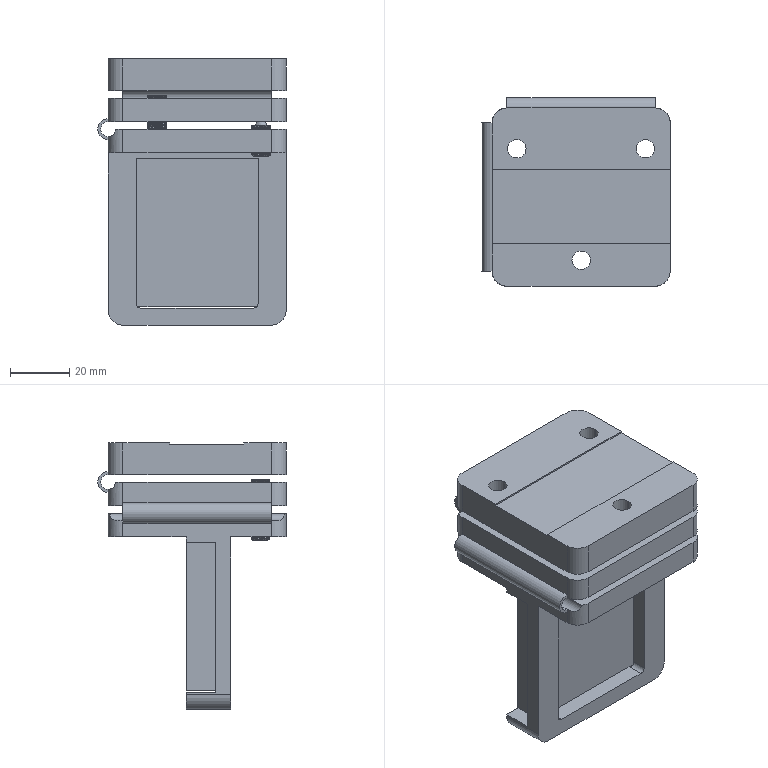Part | SolidWorks | features CompositeCurve 1 | 5 solids | 144 faces | box 63.5 x 63.5 x 89.7 mm | volume 124553 mm3 | cylinder 61 | plane 61 | cone 16 | spline 4 | sphere 2 | commonest cylinder face diameters 10 x14 12 x12 0.4 x6 3.3 x6 6.2 x6 4 x4